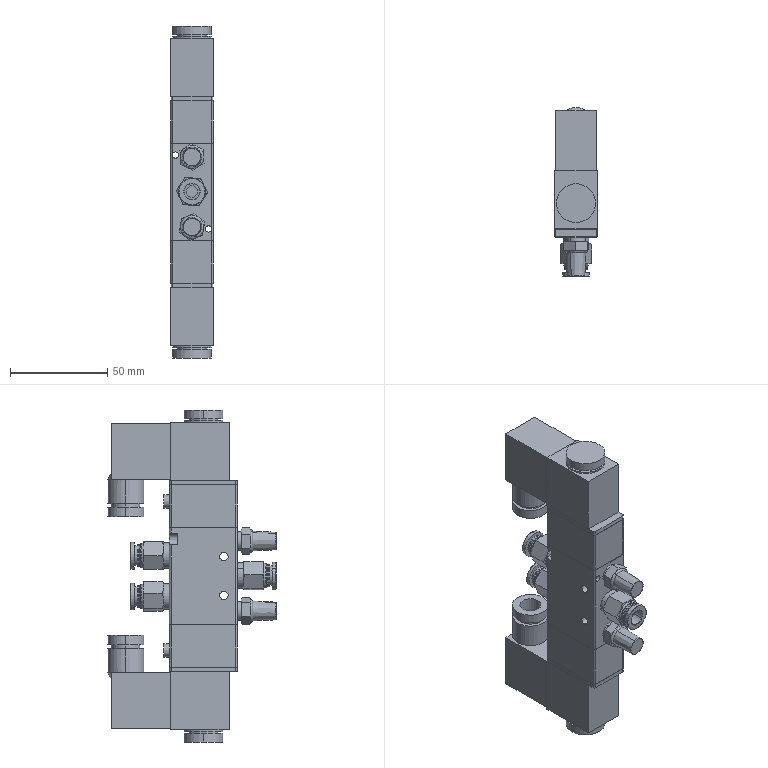Part | NX | features BREP 2 | 4 solids | 422 faces | box 22 x 86.8 x 170.8 mm | volume 168948 mm3 | plane 139 | cylinder 124 | cone 97 | torus 62 | commonest cylinder face diameters 2 x22 11.6 x12 6 x8 15 x8 18.6 x8 20 x8